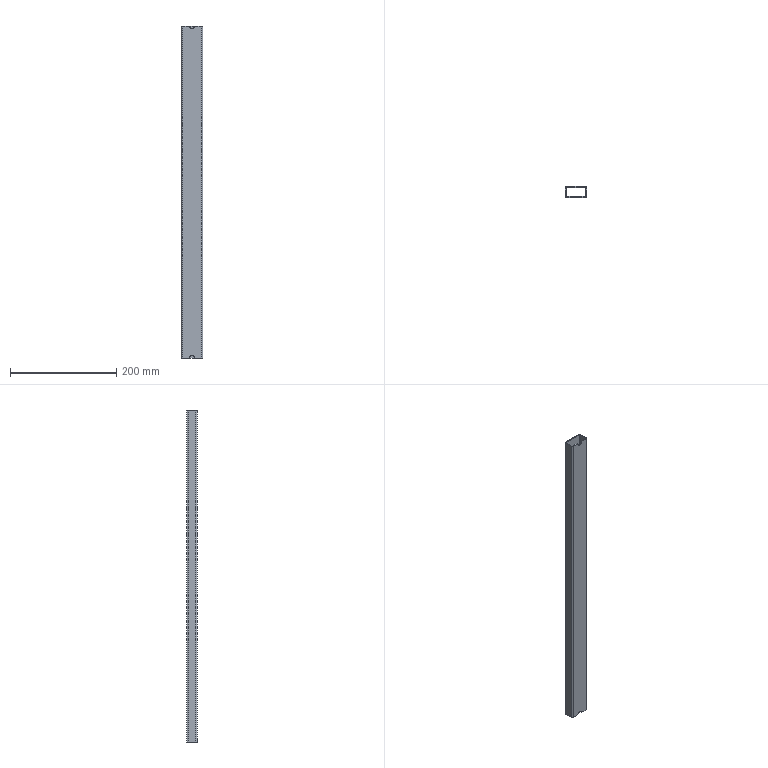Part | STEP file | 5090102 | 1 solid | 20 faces | box 40 x 20 x 624 mm | volume 103774 mm3 | plane 10 | cylinder 10 | commonest cylinder face diameters 2 x4 5 x4 10 x2